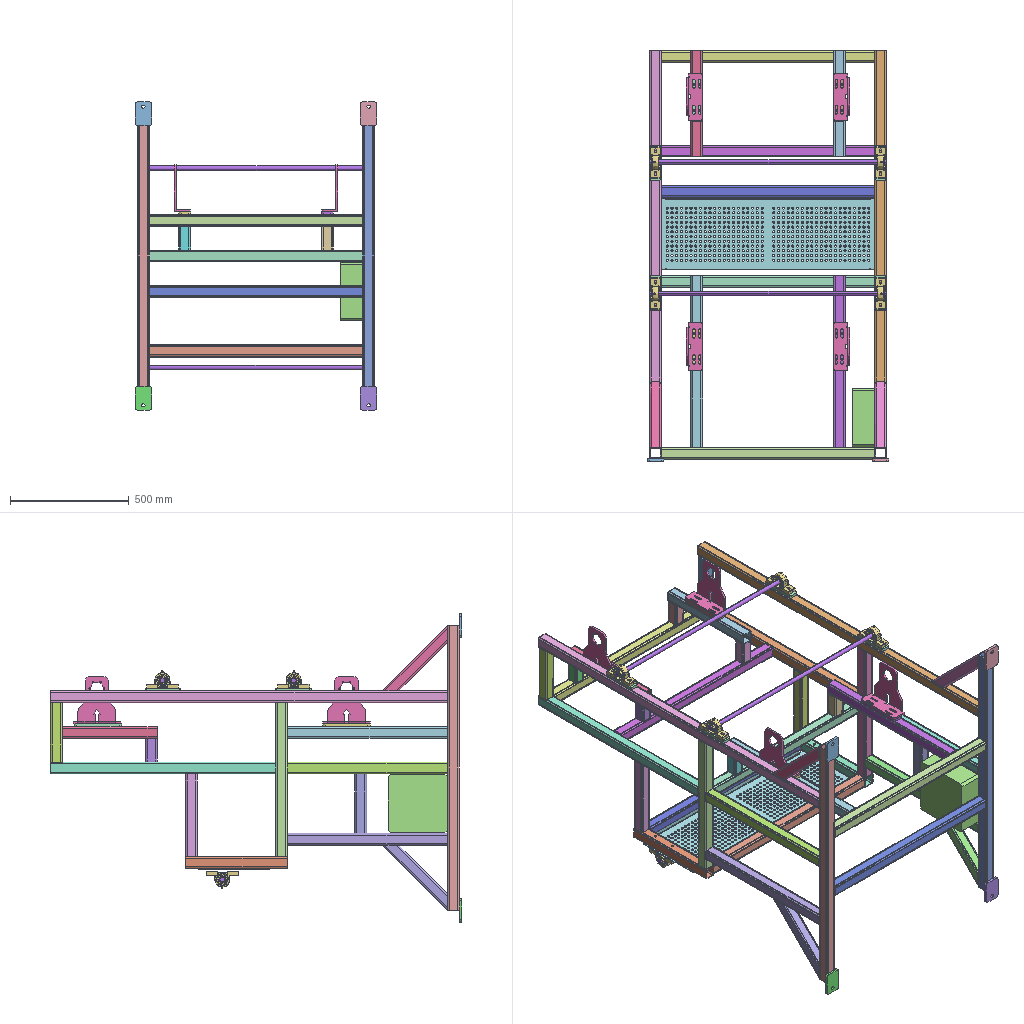Assembly | SolidWorks | 9 different items | 27 placed | box 1020 x 1735 x 1300 mm
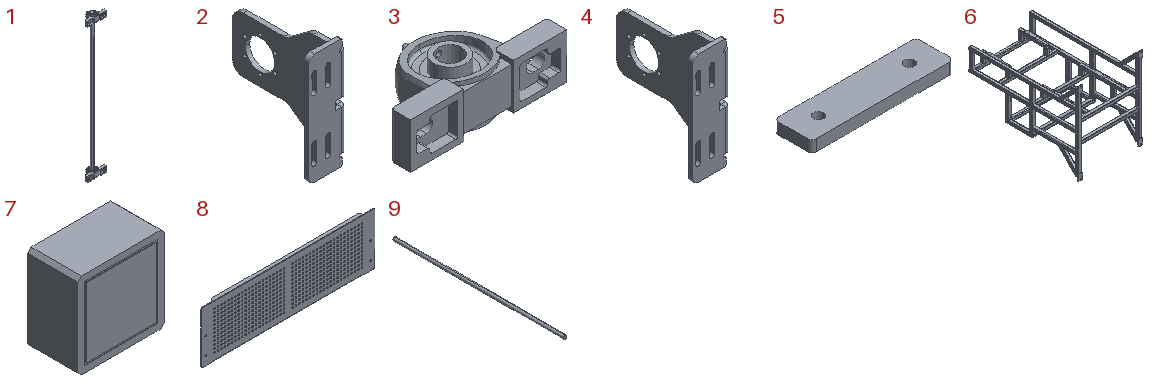Parts list (item | name | quantity | parent item | size | volume | features):
1 | (subassembly) | x3 | - | 134 x 72.66 x 1000 mm | 523004 mm3 | -
2 | (subassembly) | x4 | - | 68 x 198 x 200 mm | 249294 mm3 | -
3 | - | x6 | in 1 | 134 x 72.66 x 39.214 mm | 104404 mm3 | features Revolution 5, Cut 3, Boss 2, CirPattern 2, ICE 2, RevCut 2, Extrusion 1, RefAxis 1, SweepCut 1
4 | - | x4 | in 2 | 68 x 198 x 200 mm | 249294 mm3 | features ICE 4, Fillet 3, EdgeFlange 1, FlatPattern 1, LPattern 1, SMBaseFlange 1, SheetMetal 1
5 | - | x4 | - | 150 x 40 x 12 mm | 69462 mm3 | features Cut 1, Extrusion 1, Fillet 1, ICE 1
6 | - | x1 | - | 1020 x 1735 x 1300 mm | 17820263 mm3 | features MirrorSolid 7, WeldCornerFeat 7, ICE 3, MoveCopyBody 3, Fillet 2, WeldMemberFeat 2, 3DProfileFeature 1, Cut 1, EndCap 1, Gusset 1, HoleWzd 1, LPattern 1, MirrorPattern 1, WeldmentFeature 1
7 | - | x1 | - | 250 x 145 x 247 mm | 8920630 mm3 | features Chamfer 1, Extrusion 1, ICE 1
8 | - | x1 | - | 1000 x 20 x 300 mm | 591466 mm3 | features ICE 2, MirrorPattern 2, EdgeFlange 1, Fillet 1, FlatPattern 1, LPattern 1, SMBaseFlange 1, SheetMetal 1
9 | - | x3 | in 1 | 20 x 1000 x 20 mm | 314159 mm3 | features Extrusion 1
Mates (type | each side: item.copy, entity, surface, feature):
In the top assembly
Coincident | 6.1 face plane GB/T 6728-2002 square hollow section 50×4 | 7.1 face plane Boss-Extrude1 | 2 times
Coincident | 6.1 face plane Boss-Extrude1 | 4.1 face plane Base-Flange1
Slot | 4.1 face cylinder Cut-Extrude4 | 6.1 face cylinder M8 Tapped Hole1
Slot | 4.1 face cylinder LPattern1 | 6.1 face cylinder M8 Tapped Hole1
Coincident | 6.1 face plane LPattern1 | 4.2 face plane Base-Flange1
Slot | 4.2 face cylinder LPattern1 | 6.1 face cylinder LPattern1
Slot | 4.2 face cylinder Cut-Extrude4 | 6.1 face cylinder LPattern1
Coincident | 6.1 face plane GB/T 6728-2002 square hollow section 50×4 | 8.1 face plane Base-Flange1
Width | 6.1 face plane GB/T 6728-2002 square hollow section 50×4 | 6.1 face plane GB/T 6728-2002 square hollow section 50×4 | 8.1 face plane Base-Flange1 | 8.1 face plane Base-Flange1
Width | 6.1 face plane GB/T 6728-2002 square hollow section 50×4 | 6.1 face plane GB/T 6728-2002 square hollow section 50×4 | 3.1 face plane Boss-Extrude1 | 3.2 face plane Boss-Extrude1
Coincident | 6.1 face plane GB/T 6728-2002 square hollow section 50×4 | 5.1 face plane Boss-Extrude1
Width | 6.1 face plane GB/T 6728-2002 square hollow section 50×4 | 6.1 face plane GB/T 6728-2002 square hollow section 50×4 | 5.1 face plane Boss-Extrude1 | 5.1 face plane Boss-Extrude1
DistanceDim | 5.1 face plane Boss-Extrude1 | 6.1 face plane GB/T 6728-2002 square hollow section 50×4
Coincident | 3.1 face plane Boss-Extrude1 | 5.1 face plane Boss-Extrude1
Slot | 3.1 face cylinder Cut-Extrude3 | 5.1 face cylinder Cut-Extrude1
DistanceDim | 5.2 face plane Boss-Extrude1 | 6.1 face plane GB/T 6728-2002 square hollow section 50×4 | 2 times
Coincident | 6.1 face plane GB/T 6728-2002 square hollow section 50×4 | 5.2 face plane Boss-Extrude1
Coincident | 5.2 face plane Boss-Extrude1 | 3.3 face plane Boss-Extrude1
Slot | 5.2 face cylinder Cut-Extrude1 | 3.3 face cylinder Cut-Extrude3
Width | 6.1 face plane GB/T 6728-2002 square hollow section 50×4 | 6.1 face plane GB/T 6728-2002 square hollow section 50×4 | 7.1 face plane Boss-Extrude1 | 7.1 face plane Boss-Extrude1
Concentric | 6.1 face cylinder Cut-Extrude2 | 8.1 face cylinder Cut-Extrude2
In subassembly 1
Concentric | 3.4 face cylinder Boss-Revolve5 | 9.1 face cylinder Boss-Extrude1
Concentric | 9.1 face cylinder Boss-Extrude1 | 3.5 face cylinder Boss-Revolve5
Parallel | 3.4 face plane Boss-Extrude1 | 3.5 face plane Boss-Extrude1
DistanceDim | 3.5 face cylinder Cut-Extrude3 | 3.4 face cylinder Cut-Extrude3
Width | 9.1 face plane Boss-Extrude1 | 9.1 face plane Boss-Extrude1 | 3.4 face plane Boss-Revolve5 | 3.5 face plane Boss-Revolve5